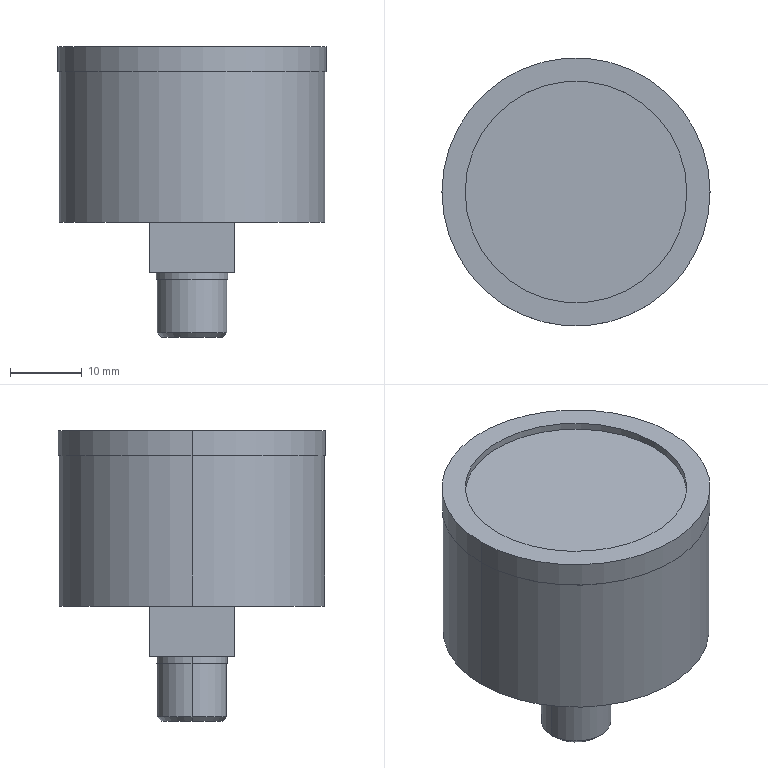Part | SolidWorks | features BaseBody 1 | 1 solid | 23 faces | box 37.5 x 37.5 x 40.6 mm | volume 27619 mm3 | plane 11 | cylinder 10 | cone 2 | commonest cylinder face diameters 9.728 x2 10 x2 31 x2 37.2 x2 37.5 x2
STEP:
#1=CARTESIAN_POINT('',(-4.283,0.,-9.1));
#2=VERTEX_POINT('',#1);
#3=CARTESIAN_POINT('',(4.283,0.,-9.1));
#4=VERTEX_POINT('',#3);
#5=CARTESIAN_POINT('',(0.,0.,-9.1));
#6=DIRECTION('',(0.,0.,-1.));
#7=DIRECTION('',(-1.,0.,0.));
#8=AXIS2_PLACEMENT_3D('',#5,#6,#7);
#9=CIRCLE('',#8,4.283);
#10=EDGE_CURVE('',#2,#4,#9,.T.);
#11=ORIENTED_EDGE('',*,*,#10,.F.);
#12=CARTESIAN_POINT('',(-4.864,0.,-8.519));
#13=VERTEX_POINT('',#12);
#14=CARTESIAN_POINT('',(-4.864,0.,-8.519));
#15=DIRECTION('',(-0.7071,0.,0.7071));
#16=VECTOR('',#15,1000.);
#17=LINE('',#14,#16);
#18=EDGE_CURVE('',#2,#13,#17,.T.);
#19=ORIENTED_EDGE('',*,*,#18,.T.);
#20=CARTESIAN_POINT('',(4.864,0.,-8.519));
#21=VERTEX_POINT('',#20);
#22=CARTESIAN_POINT('',(0.,0.,-8.519));
#23=DIRECTION('',(0.,0.,-1.));
#24=DIRECTION('',(-1.,0.,0.));
#25=AXIS2_PLACEMENT_3D('',#22,#23,#24);
#26=CIRCLE('',#25,4.864);
#27=EDGE_CURVE('',#13,#21,#26,.T.);
#28=ORIENTED_EDGE('',*,*,#27,.T.);
#29=CARTESIAN_POINT('',(4.864,0.,-8.519));
#30=DIRECTION('',(0.7071,0.,0.7071));
#31=VECTOR('',#30,1000.);
#32=LINE('',#29,#31);
#33=EDGE_CURVE('',#4,#21,#32,.T.);
#34=ORIENTED_EDGE('',*,*,#33,.F.);
#35=EDGE_LOOP('',(#11,#19,#28,#34));
#36=FACE_OUTER_BOUND('',#35,.T.);
#37=CARTESIAN_POINT('',(0.,0.,-8.519));
#38=DIRECTION('',(0.,0.,1.));
#39=DIRECTION('',(1.,0.,0.));
#40=AXIS2_PLACEMENT_3D('',#37,#38,#39);
#41=CONICAL_SURFACE('',#40,4.864,0.7854);
#42=ADVANCED_FACE('',(#36),#41,.T.);
#43=CARTESIAN_POINT('',(-4.864,0.,-1.));
#44=VERTEX_POINT('',#43);
#45=CARTESIAN_POINT('',(4.864,0.,-1.));
#46=VERTEX_POINT('',#45);
#47=CARTESIAN_POINT('',(0.,0.,-1.));
#48=DIRECTION('',(0.,0.,-1.));
#49=DIRECTION('',(-1.,0.,0.));
#50=AXIS2_PLACEMENT_3D('',#47,#48,#49);
#51=CIRCLE('',#50,4.864);
#52=EDGE_CURVE('',#44,#46,#51,.T.);
#53=ORIENTED_EDGE('',*,*,#52,.T.);
#54=CARTESIAN_POINT('',(4.864,0.,-9.1));
#55=DIRECTION('',(0.,0.,-1.));
#56=VECTOR('',#55,1000.);
#57=LINE('',#54,#56);
#58=EDGE_CURVE('',#46,#21,#57,.T.);
#59=ORIENTED_EDGE('',*,*,#58,.T.);
#60=ORIENTED_EDGE('',*,*,#27,.F.);
#61=CARTESIAN_POINT('',(-4.864,0.,-9.1));
#62=DIRECTION('',(0.,0.,-1.));
#63=VECTOR('',#62,1000.);
#64=LINE('',#61,#63);
#65=EDGE_CURVE('',#44,#13,#64,.T.);
#66=ORIENTED_EDGE('',*,*,#65,.F.);
#67=EDGE_LOOP('',(#53,#59,#60,#66));
#68=FACE_OUTER_BOUND('',#67,.T.);
#69=CARTESIAN_POINT('',(0.,0.,-9.1));
#70=DIRECTION('',(0.,0.,-1.));
#71=DIRECTION('',(-1.,0.,0.));
#72=AXIS2_PLACEMENT_3D('',#69,#70,#71);
#73=CYLINDRICAL_SURFACE('',#72,4.864);
#74=ADVANCED_FACE('',(#68),#73,.T.);
#75=CARTESIAN_POINT('',(-5.,0.,0.));
#76=VERTEX_POINT('',#75);
#77=CARTESIAN_POINT('',(5.,0.,0.));
#78=VERTEX_POINT('',#77);
#79=CARTESIAN_POINT('',(0.,0.,0.));
#80=DIRECTION('',(0.,0.,-1.));
#81=DIRECTION('',(-1.,0.,0.));
#82=AXIS2_PLACEMENT_3D('',#79,#80,#81);
#83=CIRCLE('',#82,5.);
#84=EDGE_CURVE('',#76,#78,#83,.T.);
#85=ORIENTED_EDGE('',*,*,#84,.T.);
#86=CARTESIAN_POINT('',(5.,0.,-1.));
#87=VERTEX_POINT('',#86);
#88=CARTESIAN_POINT('',(5.,0.,-9.1));
#89=DIRECTION('',(0.,0.,-1.));
#90=VECTOR('',#89,1000.);
#91=LINE('',#88,#90);
#92=EDGE_CURVE('',#78,#87,#91,.T.);
#93=ORIENTED_EDGE('',*,*,#92,.T.);
#94=CARTESIAN_POINT('',(-5.,0.,-1.));
#95=VERTEX_POINT('',#94);
#96=CARTESIAN_POINT('',(0.,0.,-1.));
#97=DIRECTION('',(0.,0.,-1.));
#98=DIRECTION('',(-1.,0.,0.));
#99=AXIS2_PLACEMENT_3D('',#96,#97,#98);
#100=CIRCLE('',#99,5.);
#101=EDGE_CURVE('',#95,#87,#100,.T.);
#102=ORIENTED_EDGE('',*,*,#101,.F.);
#103=CARTESIAN_POINT('',(-5.,0.,-9.1));
#104=DIRECTION('',(0.,0.,-1.));
#105=VECTOR('',#104,1000.);
#106=LINE('',#103,#105);
#107=EDGE_CURVE('',#76,#95,#106,.T.);
#108=ORIENTED_EDGE('',*,*,#107,.F.);
#109=EDGE_LOOP('',(#85,#93,#102,#108));
#110=FACE_OUTER_BOUND('',#109,.T.);
#111=CARTESIAN_POINT('',(0.,0.,-9.1));
#112=DIRECTION('',(0.,0.,-1.));
#113=DIRECTION('',(-1.,0.,0.));
#114=AXIS2_PLACEMENT_3D('',#111,#112,#113);
#115=CYLINDRICAL_SURFACE('',#114,5.);
#116=ADVANCED_FACE('',(#110),#115,.T.);
#117=CARTESIAN_POINT('',(-18.6,0.,28.));
#118=VERTEX_POINT('',#117);
#119=CARTESIAN_POINT('',(18.6,0.,28.));
#120=VERTEX_POINT('',#119);
#121=CARTESIAN_POINT('',(0.,0.,28.));
#122=DIRECTION('',(0.,0.,-1.));
#123=DIRECTION('',(-1.,0.,0.));
#124=AXIS2_PLACEMENT_3D('',#121,#122,#123);
#125=CIRCLE('',#124,18.6);
#126=EDGE_CURVE('',#118,#120,#125,.T.);
#127=ORIENTED_EDGE('',*,*,#126,.T.);
#128=CARTESIAN_POINT('',(18.6,0.,7.));
#129=VERTEX_POINT('',#128);
#130=CARTESIAN_POINT('',(18.6,0.,-9.1));
#131=DIRECTION('',(0.,0.,-1.));
#132=VECTOR('',#131,1000.);
#133=LINE('',#130,#132);
#134=EDGE_CURVE('',#120,#129,#133,.T.);
#135=ORIENTED_EDGE('',*,*,#134,.T.);
#136=CARTESIAN_POINT('',(-18.6,0.,7.));
#137=VERTEX_POINT('',#136);
#138=CARTESIAN_POINT('',(0.,0.,7.));
#139=DIRECTION('',(0.,0.,-1.));
#140=DIRECTION('',(-1.,0.,0.));
#141=AXIS2_PLACEMENT_3D('',#138,#139,#140);
#142=CIRCLE('',#141,18.6);
#143=EDGE_CURVE('',#137,#129,#142,.T.);
#144=ORIENTED_EDGE('',*,*,#143,.F.);
#145=CARTESIAN_POINT('',(-18.6,0.,-9.1));
#146=DIRECTION('',(0.,0.,-1.));
#147=VECTOR('',#146,1000.);
#148=LINE('',#145,#147);
#149=EDGE_CURVE('',#118,#137,#148,.T.);
#150=ORIENTED_EDGE('',*,*,#149,.F.);
#151=EDGE_LOOP('',(#127,#135,#144,#150));
#152=FACE_OUTER_BOUND('',#151,.T.);
#153=CARTESIAN_POINT('',(0.,0.,-9.1));
#154=DIRECTION('',(0.,0.,-1.));
#155=DIRECTION('',(-1.,0.,0.));
#156=AXIS2_PLACEMENT_3D('',#153,#154,#155);
#157=CYLINDRICAL_SURFACE('',#156,18.6);
#158=ADVANCED_FACE('',(#152),#157,.T.);
#159=CARTESIAN_POINT('',(-15.5,0.,30.5));
#160=VERTEX_POINT('',#159);
#161=CARTESIAN_POINT('',(15.5,0.,30.5));
#162=VERTEX_POINT('',#161);
#163=CARTESIAN_POINT('',(0.,0.,30.5));
#164=DIRECTION('',(0.,0.,1.));
#165=DIRECTION('',(0.,1.,0.));
#166=AXIS2_PLACEMENT_3D('',#163,#164,#165);
#167=CIRCLE('',#166,15.5);
#168=EDGE_CURVE('',#160,#162,#167,.T.);
#169=ORIENTED_EDGE('',*,*,#168,.F.);
#170=CARTESIAN_POINT('',(-15.5,0.,31.5));
#171=VERTEX_POINT('',#170);
#172=CARTESIAN_POINT('',(-15.5,0.,30.5));
#173=DIRECTION('',(0.,0.,1.));
#174=VECTOR('',#173,1000.);
#175=LINE('',#172,#174);
#176=EDGE_CURVE('',#160,#171,#175,.T.);
#177=ORIENTED_EDGE('',*,*,#176,.T.);
#178=CARTESIAN_POINT('',(15.5,0.,31.5));
#179=VERTEX_POINT('',#178);
#180=CARTESIAN_POINT('',(0.,0.,31.5));
#181=DIRECTION('',(0.,0.,1.));
#182=DIRECTION('',(0.,1.,0.));
#183=AXIS2_PLACEMENT_3D('',#180,#181,#182);
#184=CIRCLE('',#183,15.5);
#185=EDGE_CURVE('',#171,#179,#184,.T.);
#186=ORIENTED_EDGE('',*,*,#185,.T.);
#187=CARTESIAN_POINT('',(15.5,0.,30.5));
#188=DIRECTION('',(0.,0.,1.));
#189=VECTOR('',#188,1000.);
#190=LINE('',#187,#189);
#191=EDGE_CURVE('',#162,#179,#190,.T.);
#192=ORIENTED_EDGE('',*,*,#191,.F.);
#193=EDGE_LOOP('',(#169,#177,#186,#192));
#194=FACE_OUTER_BOUND('',#193,.T.);
#195=CARTESIAN_POINT('',(0.,0.,30.5));
#196=DIRECTION('',(0.,0.,1.));
#197=DIRECTION('',(1.,0.,0.));
#198=AXIS2_PLACEMENT_3D('',#195,#196,#197);
#199=CYLINDRICAL_SURFACE('',#198,15.5);
#200=ADVANCED_FACE('',(#194),#199,.F.);
#201=CARTESIAN_POINT('',(-18.75,0.,31.5));
#202=VERTEX_POINT('',#201);
#203=CARTESIAN_POINT('',(18.75,0.,31.5));
#204=VERTEX_POINT('',#203);
#205=CARTESIAN_POINT('',(0.,0.,31.5));
#206=DIRECTION('',(0.,0.,-1.));
#207=DIRECTION('',(-1.,0.,0.));
#208=AXIS2_PLACEMENT_3D('',#205,#206,#207);
#209=CIRCLE('',#208,18.75);
#210=EDGE_CURVE('',#202,#204,#209,.T.);
#211=ORIENTED_EDGE('',*,*,#210,.T.);
#212=CARTESIAN_POINT('',(18.75,0.,28.));
#213=VERTEX_POINT('',#212);
#214=CARTESIAN_POINT('',(18.75,0.,-9.1));
#215=DIRECTION('',(0.,0.,-1.));
#216=VECTOR('',#215,1000.);
#217=LINE('',#214,#216);
#218=EDGE_CURVE('',#204,#213,#217,.T.);
#219=ORIENTED_EDGE('',*,*,#218,.T.);
#220=CARTESIAN_POINT('',(-18.75,0.,28.));
#221=VERTEX_POINT('',#220);
#222=CARTESIAN_POINT('',(0.,0.,28.));
#223=DIRECTION('',(0.,0.,-1.));
#224=DIRECTION('',(-1.,0.,0.));
#225=AXIS2_PLACEMENT_3D('',#222,#223,#224);
#226=CIRCLE('',#225,18.75);
#227=EDGE_CURVE('',#221,#213,#226,.T.);
#228=ORIENTED_EDGE('',*,*,#227,.F.);
#229=CARTESIAN_POINT('',(-18.75,0.,-9.1));
#230=DIRECTION('',(0.,0.,-1.));
#231=VECTOR('',#230,1000.);
#232=LINE('',#229,#231);
#233=EDGE_CURVE('',#202,#221,#232,.T.);
#234=ORIENTED_EDGE('',*,*,#233,.F.);
#235=EDGE_LOOP('',(#211,#219,#228,#234));
#236=FACE_OUTER_BOUND('',#235,.T.);
#237=CARTESIAN_POINT('',(0.,0.,-9.1));
#238=DIRECTION('',(0.,0.,-1.));
#239=DIRECTION('',(-1.,0.,0.));
#240=AXIS2_PLACEMENT_3D('',#237,#238,#239);
#241=CYLINDRICAL_SURFACE('',#240,18.75);
#242=ADVANCED_FACE('',(#236),#241,.T.);
#243=ORIENTED_EDGE('',*,*,#210,.F.);
#244=CARTESIAN_POINT('',(0.,0.,31.5));
#245=DIRECTION('',(0.,0.,-1.));
#246=DIRECTION('',(-1.,0.,0.));
#247=AXIS2_PLACEMENT_3D('',#244,#245,#246);
#248=CIRCLE('',#247,18.75);
#249=EDGE_CURVE('',#204,#202,#248,.T.);
#250=ORIENTED_EDGE('',*,*,#249,.F.);
#251=EDGE_LOOP('',(#243,#250));
#252=FACE_OUTER_BOUND('',#251,.T.);
#253=CARTESIAN_POINT('',(0.,0.,31.5));
#254=DIRECTION('',(0.,0.,1.));
#255=DIRECTION('',(0.,1.,0.));
#256=AXIS2_PLACEMENT_3D('',#253,#254,#255);
#257=CIRCLE('',#256,15.5);
#258=EDGE_CURVE('',#179,#171,#257,.T.);
#259=ORIENTED_EDGE('',*,*,#258,.F.);
#260=ORIENTED_EDGE('',*,*,#185,.F.);
#261=EDGE_LOOP('',(#259,#260));
#262=FACE_BOUND('',#261,.T.);
#263=CARTESIAN_POINT('',(0.,0.,31.5));
#264=DIRECTION('',(0.,0.,-1.));
#265=DIRECTION('',(-1.,0.,0.));
#266=AXIS2_PLACEMENT_3D('',#263,#264,#265);
#267=PLANE('',#266);
#268=ADVANCED_FACE('',(#252,#262),#267,.F.);
#269=ORIENTED_EDGE('',*,*,#218,.F.);
#270=ORIENTED_EDGE('',*,*,#249,.T.);
#271=ORIENTED_EDGE('',*,*,#233,.T.);
#272=CARTESIAN_POINT('',(0.,0.,28.));
#273=DIRECTION('',(0.,0.,-1.));
#274=DIRECTION('',(-1.,0.,0.));
#275=AXIS2_PLACEMENT_3D('',#272,#273,#274);
#276=CIRCLE('',#275,18.75);
#277=EDGE_CURVE('',#213,#221,#276,.T.);
#278=ORIENTED_EDGE('',*,*,#277,.F.);
#279=EDGE_LOOP('',(#269,#270,#271,#278));
#280=FACE_OUTER_BOUND('',#279,.T.);
#281=CARTESIAN_POINT('',(0.,0.,-9.1));
#282=DIRECTION('',(0.,0.,-1.));
#283=DIRECTION('',(-1.,0.,0.));
#284=AXIS2_PLACEMENT_3D('',#281,#282,#283);
#285=CYLINDRICAL_SURFACE('',#284,18.75);
#286=ADVANCED_FACE('',(#280),#285,.T.);
#287=ORIENTED_EDGE('',*,*,#176,.F.);
#288=CARTESIAN_POINT('',(0.,0.,30.5));
#289=DIRECTION('',(0.,0.,1.));
#290=DIRECTION('',(0.,1.,0.));
#291=AXIS2_PLACEMENT_3D('',#288,#289,#290);
#292=CIRCLE('',#291,15.5);
#293=EDGE_CURVE('',#162,#160,#292,.T.);
#294=ORIENTED_EDGE('',*,*,#293,.F.);
#295=ORIENTED_EDGE('',*,*,#191,.T.);
#296=ORIENTED_EDGE('',*,*,#258,.T.);
#297=EDGE_LOOP('',(#287,#294,#295,#296));
#298=FACE_OUTER_BOUND('',#297,.T.);
#299=CARTESIAN_POINT('',(0.,0.,30.5));
#300=DIRECTION('',(0.,0.,1.));
#301=DIRECTION('',(1.,0.,0.));
#302=AXIS2_PLACEMENT_3D('',#299,#300,#301);
#303=CYLINDRICAL_SURFACE('',#302,15.5);
#304=ADVANCED_FACE('',(#298),#303,.F.);
#305=ORIENTED_EDGE('',*,*,#126,.F.);
#306=CARTESIAN_POINT('',(0.,0.,28.));
#307=DIRECTION('',(0.,0.,-1.));
#308=DIRECTION('',(-1.,0.,0.));
#309=AXIS2_PLACEMENT_3D('',#306,#307,#308);
#310=CIRCLE('',#309,18.6);
#311=EDGE_CURVE('',#120,#118,#310,.T.);
#312=ORIENTED_EDGE('',*,*,#311,.F.);
#313=EDGE_LOOP('',(#305,#312));
#314=FACE_BOUND('',#313,.T.);
#315=ORIENTED_EDGE('',*,*,#227,.T.);
#316=ORIENTED_EDGE('',*,*,#277,.T.);
#317=EDGE_LOOP('',(#315,#316));
#318=FACE_OUTER_BOUND('',#317,.T.);
#319=CARTESIAN_POINT('',(0.,18.75,28.));
#320=DIRECTION('',(0.,0.,1.));
#321=DIRECTION('',(1.,0.,0.));
#322=AXIS2_PLACEMENT_3D('',#319,#320,#321);
#323=PLANE('',#322);
#324=ADVANCED_FACE('',(#314,#318),#323,.F.);
#325=ORIENTED_EDGE('',*,*,#293,.T.);
#326=ORIENTED_EDGE('',*,*,#168,.T.);
#327=EDGE_LOOP('',(#325,#326));
#328=FACE_OUTER_BOUND('',#327,.T.);
#329=CARTESIAN_POINT('',(0.,0.,30.5));
#330=DIRECTION('',(0.,0.,1.));
#331=DIRECTION('',(1.,0.,0.));
#332=AXIS2_PLACEMENT_3D('',#329,#330,#331);
#333=PLANE('',#332);
#334=ADVANCED_FACE('',(#328),#333,.T.);
#335=ORIENTED_EDGE('',*,*,#134,.F.);
#336=ORIENTED_EDGE('',*,*,#311,.T.);
#337=ORIENTED_EDGE('',*,*,#149,.T.);
#338=CARTESIAN_POINT('',(0.,0.,7.));
#339=DIRECTION('',(0.,0.,-1.));
#340=DIRECTION('',(-1.,0.,0.));
#341=AXIS2_PLACEMENT_3D('',#338,#339,#340);
#342=CIRCLE('',#341,18.6);
#343=EDGE_CURVE('',#129,#137,#342,.T.);
#344=ORIENTED_EDGE('',*,*,#343,.F.);
#345=EDGE_LOOP('',(#335,#336,#337,#344));
#346=FACE_OUTER_BOUND('',#345,.T.);
#347=CARTESIAN_POINT('',(0.,0.,-9.1));
#348=DIRECTION('',(0.,0.,-1.));
#349=DIRECTION('',(-1.,0.,0.));
#350=AXIS2_PLACEMENT_3D('',#347,#348,#349);
#351=CYLINDRICAL_SURFACE('',#350,18.6);
#352=ADVANCED_FACE('',(#346),#351,.T.);
#353=ORIENTED_EDGE('',*,*,#143,.T.);
#354=ORIENTED_EDGE('',*,*,#343,.T.);
#355=EDGE_LOOP('',(#353,#354));
#356=FACE_OUTER_BOUND('',#355,.T.);
#357=CARTESIAN_POINT('',(6.,-6.,7.));
#358=VERTEX_POINT('',#357);
#359=CARTESIAN_POINT('',(-6.,-6.,7.));
#360=VERTEX_POINT('',#359);
#361=CARTESIAN_POINT('',(6.,-6.,7.));
#362=DIRECTION('',(-1.,0.,0.));
#363=VECTOR('',#362,1000.);
#364=LINE('',#361,#363);
#365=EDGE_CURVE('',#358,#360,#364,.T.);
#366=ORIENTED_EDGE('',*,*,#365,.F.);
#367=CARTESIAN_POINT('',(6.,6.,7.));
#368=VERTEX_POINT('',#367);
#369=CARTESIAN_POINT('',(6.,6.,7.));
#370=DIRECTION('',(0.,-1.,0.));
#371=VECTOR('',#370,1000.);
#372=LINE('',#369,#371);
#373=EDGE_CURVE('',#368,#358,#372,.T.);
#374=ORIENTED_EDGE('',*,*,#373,.F.);
#375=CARTESIAN_POINT('',(-6.,6.,7.));
#376=VERTEX_POINT('',#375);
#377=CARTESIAN_POINT('',(-6.,6.,7.));
#378=DIRECTION('',(1.,0.,0.));
#379=VECTOR('',#378,1000.);
#380=LINE('',#377,#379);
#381=EDGE_CURVE('',#376,#368,#380,.T.);
#382=ORIENTED_EDGE('',*,*,#381,.F.);
#383=CARTESIAN_POINT('',(-6.,-6.,7.));
#384=DIRECTION('',(0.,1.,0.));
#385=VECTOR('',#384,1000.);
#386=LINE('',#383,#385);
#387=EDGE_CURVE('',#360,#376,#386,.T.);
#388=ORIENTED_EDGE('',*,*,#387,.F.);
#389=EDGE_LOOP('',(#366,#374,#382,#388));
#390=FACE_BOUND('',#389,.T.);
#391=CARTESIAN_POINT('',(0.,18.6,7.));
#392=DIRECTION('',(0.,0.,1.));
#393=DIRECTION('',(1.,0.,0.));
#394=AXIS2_PLACEMENT_3D('',#391,#392,#393);
#395=PLANE('',#394);
#396=ADVANCED_FACE('',(#356,#390),#395,.F.);
#397=CARTESIAN_POINT('',(6.,-6.,0.));
#398=VERTEX_POINT('',#397);
#399=CARTESIAN_POINT('',(-6.,-6.,0.));
#400=VERTEX_POINT('',#399);
#401=CARTESIAN_POINT('',(6.,-6.,0.));
#402=DIRECTION('',(-1.,0.,0.));
#403=VECTOR('',#402,1000.);
#404=LINE('',#401,#403);
#405=EDGE_CURVE('',#398,#400,#404,.T.);
#406=ORIENTED_EDGE('',*,*,#405,.F.);
#407=CARTESIAN_POINT('',(6.,-6.,7.));
#408=DIRECTION('',(0.,0.,-1.));
#409=VECTOR('',#408,1000.);
#410=LINE('',#407,#409);
#411=EDGE_CURVE('',#358,#398,#410,.T.);
#412=ORIENTED_EDGE('',*,*,#411,.F.);
#413=ORIENTED_EDGE('',*,*,#365,.T.);
#414=CARTESIAN_POINT('',(-6.,-6.,7.));
#415=DIRECTION('',(0.,0.,-1.));
#416=VECTOR('',#415,1000.);
#417=LINE('',#414,#416);
#418=EDGE_CURVE('',#360,#400,#417,.T.);
#419=ORIENTED_EDGE('',*,*,#418,.T.);
#420=EDGE_LOOP('',(#406,#412,#413,#419));
#421=FACE_OUTER_BOUND('',#420,.T.);
#422=CARTESIAN_POINT('',(6.,-6.,7.));
#423=DIRECTION('',(0.,-1.,0.));
#424=DIRECTION('',(0.,0.,-1.));
#425=AXIS2_PLACEMENT_3D('',#422,#423,#424);
#426=PLANE('',#425);
#427=ADVANCED_FACE('',(#421),#426,.T.);
#428=CARTESIAN_POINT('',(6.,6.,0.));
#429=VERTEX_POINT('',#428);
#430=CARTESIAN_POINT('',(6.,6.,0.));
#431=DIRECTION('',(0.,-1.,0.));
#432=VECTOR('',#431,1000.);
#433=LINE('',#430,#432);
#434=EDGE_CURVE('',#429,#398,#433,.T.);
#435=ORIENTED_EDGE('',*,*,#434,.F.);
#436=CARTESIAN_POINT('',(6.,6.,7.));
#437=DIRECTION('',(0.,0.,-1.));
#438=VECTOR('',#437,1000.);
#439=LINE('',#436,#438);
#440=EDGE_CURVE('',#368,#429,#439,.T.);
#441=ORIENTED_EDGE('',*,*,#440,.F.);
#442=ORIENTED_EDGE('',*,*,#373,.T.);
#443=ORIENTED_EDGE('',*,*,#411,.T.);
#444=EDGE_LOOP('',(#435,#441,#442,#443));
#445=FACE_OUTER_BOUND('',#444,.T.);
#446=CARTESIAN_POINT('',(6.,6.,7.));
#447=DIRECTION('',(1.,0.,0.));
#448=DIRECTION('',(0.,0.,-1.));
#449=AXIS2_PLACEMENT_3D('',#446,#447,#448);
#450=PLANE('',#449);
#451=ADVANCED_FACE('',(#445),#450,.T.);
#452=CARTESIAN_POINT('',(-6.,6.,0.));
#453=VERTEX_POINT('',#452);
#454=CARTESIAN_POINT('',(6.,6.,0.));
#455=DIRECTION('',(-1.,0.,0.));
#456=VECTOR('',#455,1000.);
#457=LINE('',#454,#456);
#458=EDGE_CURVE('',#429,#453,#457,.T.);
#459=ORIENTED_EDGE('',*,*,#458,.T.);
#460=CARTESIAN_POINT('',(-6.,6.,7.));
#461=DIRECTION('',(0.,0.,-1.));
#462=VECTOR('',#461,1000.);
#463=LINE('',#460,#462);
#464=EDGE_CURVE('',#376,#453,#463,.T.);
#465=ORIENTED_EDGE('',*,*,#464,.F.);
#466=ORIENTED_EDGE('',*,*,#381,.T.);
#467=ORIENTED_EDGE('',*,*,#440,.T.);
#468=EDGE_LOOP('',(#459,#465,#466,#467));
#469=FACE_OUTER_BOUND('',#468,.T.);
#470=CARTESIAN_POINT('',(-6.,6.,7.));
#471=DIRECTION('',(0.,1.,0.));
#472=DIRECTION('',(0.,0.,1.));
#473=AXIS2_PLACEMENT_3D('',#470,#471,#472);
#474=PLANE('',#473);
#475=ADVANCED_FACE('',(#469),#474,.T.);
#476=CARTESIAN_POINT('',(-6.,-6.,0.));
#477=DIRECTION('',(0.,1.,0.));
#478=VECTOR('',#477,1000.);
#479=LINE('',#476,#478);
#480=EDGE_CURVE('',#400,#453,#479,.T.);
#481=ORIENTED_EDGE('',*,*,#480,.F.);
#482=ORIENTED_EDGE('',*,*,#418,.F.);
#483=ORIENTED_EDGE('',*,*,#387,.T.);
#484=ORIENTED_EDGE('',*,*,#464,.T.);
#485=EDGE_LOOP('',(#481,#482,#483,#484));
#486=FACE_OUTER_BOUND('',#485,.T.);
#487=CARTESIAN_POINT('',(-6.,-6.,7.));
#488=DIRECTION('',(-1.,0.,0.));
#489=DIRECTION('',(0.,0.,1.));
#490=AXIS2_PLACEMENT_3D('',#487,#488,#489);
#491=PLANE('',#490);
#492=ADVANCED_FACE('',(#486),#491,.T.);
#493=ORIENTED_EDGE('',*,*,#84,.F.);
#494=CARTESIAN_POINT('',(0.,0.,0.));
#495=DIRECTION('',(0.,0.,-1.));
#496=DIRECTION('',(-1.,0.,0.));
#497=AXIS2_PLACEMENT_3D('',#494,#495,#496);
#498=CIRCLE('',#497,5.);
#499=EDGE_CURVE('',#78,#76,#498,.T.);
#500=ORIENTED_EDGE('',*,*,#499,.F.);
#501=EDGE_LOOP('',(#493,#500));
#502=FACE_BOUND('',#501,.T.);
#503=ORIENTED_EDGE('',*,*,#405,.T.);
#504=ORIENTED_EDGE('',*,*,#480,.T.);
#505=ORIENTED_EDGE('',*,*,#458,.F.);
#506=ORIENTED_EDGE('',*,*,#434,.T.);
#507=EDGE_LOOP('',(#503,#504,#505,#506));
#508=FACE_OUTER_BOUND('',#507,.T.);
#509=CARTESIAN_POINT('',(0.,15.,0.));
#510=DIRECTION('',(0.,0.,1.));
#511=DIRECTION('',(1.,0.,0.));
#512=AXIS2_PLACEMENT_3D('',#509,#510,#511);
#513=PLANE('',#512);
#514=ADVANCED_FACE('',(#502,#508),#513,.F.);
#515=ORIENTED_EDGE('',*,*,#92,.F.);
#516=ORIENTED_EDGE('',*,*,#499,.T.);
#517=ORIENTED_EDGE('',*,*,#107,.T.);
#518=CARTESIAN_POINT('',(0.,0.,-1.));
#519=DIRECTION('',(0.,0.,-1.));
#520=DIRECTION('',(-1.,0.,0.));
#521=AXIS2_PLACEMENT_3D('',#518,#519,#520);
#522=CIRCLE('',#521,5.);
#523=EDGE_CURVE('',#87,#95,#522,.T.);
#524=ORIENTED_EDGE('',*,*,#523,.F.);
#525=EDGE_LOOP('',(#515,#516,#517,#524));
#526=FACE_OUTER_BOUND('',#525,.T.);
#527=CARTESIAN_POINT('',(0.,0.,-9.1));
#528=DIRECTION('',(0.,0.,-1.));
#529=DIRECTION('',(-1.,0.,0.));
#530=AXIS2_PLACEMENT_3D('',#527,#528,#529);
#531=CYLINDRICAL_SURFACE('',#530,5.);
#532=ADVANCED_FACE('',(#526),#531,.T.);
#533=ORIENTED_EDGE('',*,*,#52,.F.);
#534=CARTESIAN_POINT('',(0.,0.,-1.));
#535=DIRECTION('',(0.,0.,-1.));
#536=DIRECTION('',(-1.,0.,0.));
#537=AXIS2_PLACEMENT_3D('',#534,#535,#536);
#538=CIRCLE('',#537,4.864);
#539=EDGE_CURVE('',#46,#44,#538,.T.);
#540=ORIENTED_EDGE('',*,*,#539,.F.);
#541=EDGE_LOOP('',(#533,#540));
#542=FACE_BOUND('',#541,.T.);
#543=ORIENTED_EDGE('',*,*,#101,.T.);
#544=ORIENTED_EDGE('',*,*,#523,.T.);
#545=EDGE_LOOP('',(#543,#544));
#546=FACE_OUTER_BOUND('',#545,.T.);
#547=CARTESIAN_POINT('',(0.,5.,-1.));
#548=DIRECTION('',(0.,0.,1.));
#549=DIRECTION('',(1.,0.,0.));
#550=AXIS2_PLACEMENT_3D('',#547,#548,#549);
#551=PLANE('',#550);
#552=ADVANCED_FACE('',(#542,#546),#551,.F.);
#553=ORIENTED_EDGE('',*,*,#58,.F.);
#554=ORIENTED_EDGE('',*,*,#539,.T.);
#555=ORIENTED_EDGE('',*,*,#65,.T.);
#556=CARTESIAN_POINT('',(0.,0.,-8.519));
#557=DIRECTION('',(0.,0.,-1.));
#558=DIRECTION('',(-1.,0.,0.));
#559=AXIS2_PLACEMENT_3D('',#556,#557,#558);
#560=CIRCLE('',#559,4.864);
#561=EDGE_CURVE('',#21,#13,#560,.T.);
#562=ORIENTED_EDGE('',*,*,#561,.F.);
#563=EDGE_LOOP('',(#553,#554,#555,#562));
#564=FACE_OUTER_BOUND('',#563,.T.);
#565=CARTESIAN_POINT('',(0.,0.,-9.1));
#566=DIRECTION('',(0.,0.,-1.));
#567=DIRECTION('',(-1.,0.,0.));
#568=AXIS2_PLACEMENT_3D('',#565,#566,#567);
#569=CYLINDRICAL_SURFACE('',#568,4.864);
#570=ADVANCED_FACE('',(#564),#569,.T.);
#571=ORIENTED_EDGE('',*,*,#18,.F.);
#572=CARTESIAN_POINT('',(0.,0.,-9.1));
#573=DIRECTION('',(0.,0.,-1.));
#574=DIRECTION('',(-1.,0.,0.));
#575=AXIS2_PLACEMENT_3D('',#572,#573,#574);
#576=CIRCLE('',#575,4.283);
#577=EDGE_CURVE('',#4,#2,#576,.T.);
#578=ORIENTED_EDGE('',*,*,#577,.F.);
#579=ORIENTED_EDGE('',*,*,#33,.T.);
#580=ORIENTED_EDGE('',*,*,#561,.T.);
#581=EDGE_LOOP('',(#571,#578,#579,#580));
#582=FACE_OUTER_BOUND('',#581,.T.);
#583=CARTESIAN_POINT('',(0.,0.,-8.519));
#584=DIRECTION('',(0.,0.,1.));
#585=DIRECTION('',(1.,0.,0.));
#586=AXIS2_PLACEMENT_3D('',#583,#584,#585);
#587=CONICAL_SURFACE('',#586,4.864,0.7854);
#588=ADVANCED_FACE('',(#582),#587,.T.);
#589=ORIENTED_EDGE('',*,*,#577,.T.);
#590=ORIENTED_EDGE('',*,*,#10,.T.);
#591=EDGE_LOOP('',(#589,#590));
#592=FACE_OUTER_BOUND('',#591,.T.);
#593=CARTESIAN_POINT('',(0.,4.283,-9.1));
#594=DIRECTION('',(0.,0.,1.));
#595=DIRECTION('',(1.,0.,0.));
#596=AXIS2_PLACEMENT_3D('',#593,#594,#595);
#597=PLANE('',#596);
#598=ADVANCED_FACE('',(#592),#597,.F.);
#599=CLOSED_SHELL('',(#42,#74,#116,#158,#200,#242,#268,#286,#304,#324,#334,#352,#396,#427,#451,#475,#492,#514,#532,#552,#570,#588,#598));
#600=MANIFOLD_SOLID_BREP('',#599);
#601=CARTESIAN_POINT('',(0.,0.,0.));
#602=DIRECTION('',(0.,0.,1.));
#603=DIRECTION('',(1.,0.,0.));
#604=AXIS2_PLACEMENT_3D('',#601,#602,#603);
#605=(LENGTH_UNIT()NAMED_UNIT(*)SI_UNIT(.MILLI.,.METRE.));
#606=UNCERTAINTY_MEASURE_WITH_UNIT(LENGTH_MEASURE(0.00001),#605,'','');
#607=(NAMED_UNIT(*)PLANE_ANGLE_UNIT()SI_UNIT($,.RADIAN.));
#608=(NAMED_UNIT(*)SI_UNIT($,.STERADIAN.)SOLID_ANGLE_UNIT());
#609=(GEOMETRIC_REPRESENTATION_CONTEXT(3)GLOBAL_UNCERTAINTY_ASSIGNED_CONTEXT((#606))GLOBAL_UNIT_ASSIGNED_CONTEXT((#605,#607,#608))REPRESENTATION_CONTEXT('',''));
#610=ADVANCED_BREP_SHAPE_REPRESENTATION('',(#600,#604),#609);